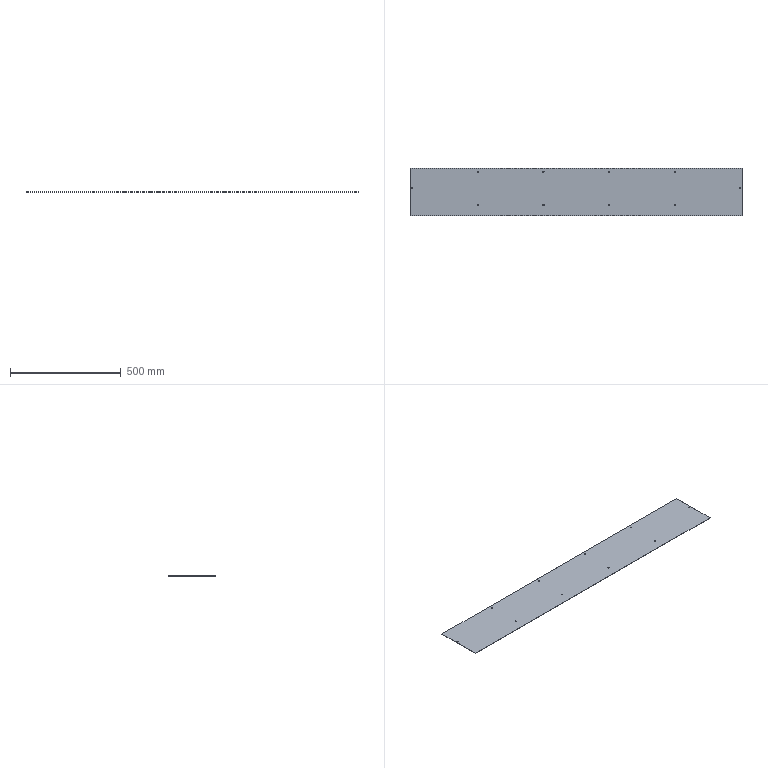Part | STEP file | SX-S23 | 1 solid | 26 faces | box 1498 x 213 x 1.2 mm | volume 382614 mm3 | cylinder 20 | plane 6 | commonest cylinder face diameters 5.4 x20